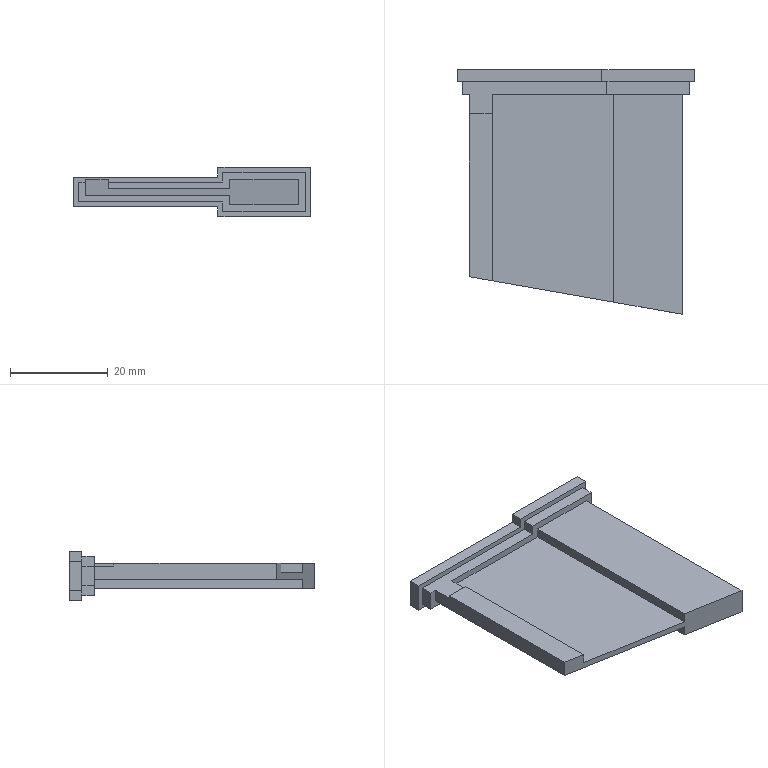Part | SolidWorks | features ICE 4, Extrusion 1 | 1 solid | 31 faces | box 48.36 x 50 x 10.06 mm | volume 6665 mm3 | plane 31
STEP:
#1=CARTESIAN_POINT('',(-43.58,41.,-0.61));
#2=VERTEX_POINT('',#1);
#3=CARTESIAN_POINT('',(-43.58,41.,0.));
#4=VERTEX_POINT('',#3);
#5=CARTESIAN_POINT('',(-43.58,41.,-0.61));
#6=DIRECTION('',(0.,0.,1.));
#7=VECTOR('',#6,1000.);
#8=LINE('',#5,#7);
#9=EDGE_CURVE('',#2,#4,#8,.T.);
#10=ORIENTED_EDGE('',*,*,#9,.F.);
#11=CARTESIAN_POINT('',(-43.58,45.,-0.61));
#12=VERTEX_POINT('',#11);
#13=CARTESIAN_POINT('',(-43.58,45.,-0.61));
#14=DIRECTION('',(0.,-1.,0.));
#15=VECTOR('',#14,1000.);
#16=LINE('',#13,#15);
#17=EDGE_CURVE('',#12,#2,#16,.T.);
#18=ORIENTED_EDGE('',*,*,#17,.F.);
#19=CARTESIAN_POINT('',(-43.58,45.,-3.28));
#20=VERTEX_POINT('',#19);
#21=CARTESIAN_POINT('',(-43.58,45.,-3.28));
#22=DIRECTION('',(0.,0.,1.));
#23=VECTOR('',#22,1000.);
#24=LINE('',#21,#23);
#25=EDGE_CURVE('',#20,#12,#24,.T.);
#26=ORIENTED_EDGE('',*,*,#25,.F.);
#27=CARTESIAN_POINT('',(-43.58,7.684,-3.28));
#28=VERTEX_POINT('',#27);
#29=CARTESIAN_POINT('',(-43.58,45.,-3.28));
#30=DIRECTION('',(0.,-1.,0.));
#31=VECTOR('',#30,1000.);
#32=LINE('',#29,#31);
#33=EDGE_CURVE('',#20,#28,#32,.T.);
#34=ORIENTED_EDGE('',*,*,#33,.T.);
#35=CARTESIAN_POINT('',(-43.58,7.684,0.));
#36=VERTEX_POINT('',#35);
#37=CARTESIAN_POINT('',(-43.58,7.684,-5.28));
#38=DIRECTION('',(0.,0.,1.));
#39=VECTOR('',#38,1000.);
#40=LINE('',#37,#39);
#41=EDGE_CURVE('',#28,#36,#40,.T.);
#42=ORIENTED_EDGE('',*,*,#41,.T.);
#43=CARTESIAN_POINT('',(-43.58,45.,0.));
#44=DIRECTION('',(0.,-1.,0.));
#45=VECTOR('',#44,1000.);
#46=LINE('',#43,#45);
#47=EDGE_CURVE('',#4,#36,#46,.T.);
#48=ORIENTED_EDGE('',*,*,#47,.F.);
#49=EDGE_LOOP('',(#10,#18,#26,#34,#42,#48));
#50=FACE_OUTER_BOUND('',#49,.T.);
#51=CARTESIAN_POINT('',(-43.58,45.,-3.28));
#52=DIRECTION('',(1.,0.,0.));
#53=DIRECTION('',(0.,0.,-1.));
#54=AXIS2_PLACEMENT_3D('',#51,#52,#53);
#55=PLANE('',#54);
#56=ADVANCED_FACE('',(#50),#55,.F.);
#57=CARTESIAN_POINT('',(-38.89,41.,0.));
#58=VERTEX_POINT('',#57);
#59=CARTESIAN_POINT('',(-38.89,6.857,0.));
#60=VERTEX_POINT('',#59);
#61=CARTESIAN_POINT('',(-38.89,45.,0.));
#62=DIRECTION('',(0.,-1.,0.));
#63=VECTOR('',#62,1000.);
#64=LINE('',#61,#63);
#65=EDGE_CURVE('',#58,#60,#64,.T.);
#66=ORIENTED_EDGE('',*,*,#65,.F.);
#67=CARTESIAN_POINT('',(-33.58,41.,0.));
#68=DIRECTION('',(-1.,0.,0.));
#69=VECTOR('',#68,1000.);
#70=LINE('',#67,#69);
#71=EDGE_CURVE('',#58,#4,#70,.T.);
#72=ORIENTED_EDGE('',*,*,#71,.T.);
#73=ORIENTED_EDGE('',*,*,#47,.T.);
#74=CARTESIAN_POINT('',(-43.58,7.684,0.));
#75=DIRECTION('',(-0.9848,0.1736,0.));
#76=VECTOR('',#75,1000.);
#77=LINE('',#74,#76);
#78=EDGE_CURVE('',#60,#36,#77,.T.);
#79=ORIENTED_EDGE('',*,*,#78,.F.);
#80=EDGE_LOOP('',(#66,#72,#73,#79));
#81=FACE_OUTER_BOUND('',#80,.T.);
#82=CARTESIAN_POINT('',(-43.58,45.,0.));
#83=DIRECTION('',(0.,0.,-1.));
#84=DIRECTION('',(-1.,0.,0.));
#85=AXIS2_PLACEMENT_3D('',#82,#83,#84);
#86=PLANE('',#85);
#87=ADVANCED_FACE('',(#81),#86,.F.);
#88=CARTESIAN_POINT('',(-38.89,45.,-0.61));
#89=VERTEX_POINT('',#88);
#90=CARTESIAN_POINT('',(-38.89,45.,-2.));
#91=VERTEX_POINT('',#90);
#92=CARTESIAN_POINT('',(-38.89,45.,0.));
#93=DIRECTION('',(0.,0.,-1.));
#94=VECTOR('',#93,1000.);
#95=LINE('',#92,#94);
#96=EDGE_CURVE('',#89,#91,#95,.T.);
#97=ORIENTED_EDGE('',*,*,#96,.F.);
#98=CARTESIAN_POINT('',(-38.89,41.,-0.61));
#99=VERTEX_POINT('',#98);
#100=CARTESIAN_POINT('',(-38.89,45.,-0.61));
#101=DIRECTION('',(0.,-1.,0.));
#102=VECTOR('',#101,1000.);
#103=LINE('',#100,#102);
#104=EDGE_CURVE('',#89,#99,#103,.T.);
#105=ORIENTED_EDGE('',*,*,#104,.T.);
#106=CARTESIAN_POINT('',(-38.89,41.,0.));
#107=DIRECTION('',(0.,0.,1.));
#108=VECTOR('',#107,1000.);
#109=LINE('',#106,#108);
#110=EDGE_CURVE('',#99,#58,#109,.T.);
#111=ORIENTED_EDGE('',*,*,#110,.T.);
#112=ORIENTED_EDGE('',*,*,#65,.T.);
#113=CARTESIAN_POINT('',(-38.89,6.857,-2.));
#114=VERTEX_POINT('',#113);
#115=CARTESIAN_POINT('',(-38.89,6.857,0.));
#116=DIRECTION('',(0.,0.,-1.));
#117=VECTOR('',#116,1000.);
#118=LINE('',#115,#117);
#119=EDGE_CURVE('',#60,#114,#118,.T.);
#120=ORIENTED_EDGE('',*,*,#119,.T.);
#121=CARTESIAN_POINT('',(-38.89,45.,-2.));
#122=DIRECTION('',(0.,-1.,0.));
#123=VECTOR('',#122,1000.);
#124=LINE('',#121,#123);
#125=EDGE_CURVE('',#91,#114,#124,.T.);
#126=ORIENTED_EDGE('',*,*,#125,.F.);
#127=EDGE_LOOP('',(#97,#105,#111,#112,#120,#126));
#128=FACE_OUTER_BOUND('',#127,.T.);
#129=CARTESIAN_POINT('',(-38.89,45.,0.));
#130=DIRECTION('',(-1.,0.,0.));
#131=DIRECTION('',(0.,0.,1.));
#132=AXIS2_PLACEMENT_3D('',#129,#130,#131);
#133=PLANE('',#132);
#134=ADVANCED_FACE('',(#128),#133,.F.);
#135=ORIENTED_EDGE('',*,*,#125,.T.);
#136=CARTESIAN_POINT('',(-14.09,2.484,-2.));
#137=VERTEX_POINT('',#136);
#138=CARTESIAN_POINT('',(-45.413,8.007,-2.));
#139=DIRECTION('',(0.9848,-0.1736,0.));
#140=VECTOR('',#139,1000.);
#141=LINE('',#138,#140);
#142=EDGE_CURVE('',#114,#137,#141,.T.);
#143=ORIENTED_EDGE('',*,*,#142,.T.);
#144=CARTESIAN_POINT('',(-14.09,45.,-2.));
#145=VERTEX_POINT('',#144);
#146=CARTESIAN_POINT('',(-14.09,45.,-2.));
#147=DIRECTION('',(0.,-1.,0.));
#148=VECTOR('',#147,1000.);
#149=LINE('',#146,#148);
#150=EDGE_CURVE('',#145,#137,#149,.T.);
#151=ORIENTED_EDGE('',*,*,#150,.F.);
#152=CARTESIAN_POINT('',(-38.89,45.,-2.));
#153=DIRECTION('',(1.,0.,0.));
#154=VECTOR('',#153,1000.);
#155=LINE('',#152,#154);
#156=EDGE_CURVE('',#91,#145,#155,.T.);
#157=ORIENTED_EDGE('',*,*,#156,.F.);
#158=EDGE_LOOP('',(#135,#143,#151,#157));
#159=FACE_OUTER_BOUND('',#158,.T.);
#160=CARTESIAN_POINT('',(-38.89,45.,-2.));
#161=DIRECTION('',(0.,0.,-1.));
#162=DIRECTION('',(-1.,0.,0.));
#163=AXIS2_PLACEMENT_3D('',#160,#161,#162);
#164=PLANE('',#163);
#165=ADVANCED_FACE('',(#159),#164,.F.);
#166=ORIENTED_EDGE('',*,*,#150,.T.);
#167=CARTESIAN_POINT('',(-14.09,2.484,0.));
#168=VERTEX_POINT('',#167);
#169=CARTESIAN_POINT('',(-14.09,2.484,-2.));
#170=DIRECTION('',(0.,0.,1.));
#171=VECTOR('',#170,1000.);
#172=LINE('',#169,#171);
#173=EDGE_CURVE('',#137,#168,#172,.T.);
#174=ORIENTED_EDGE('',*,*,#173,.T.);
#175=CARTESIAN_POINT('',(-14.09,45.,0.));
#176=VERTEX_POINT('',#175);
#177=CARTESIAN_POINT('',(-14.09,45.,0.));
#178=DIRECTION('',(0.,-1.,0.));
#179=VECTOR('',#178,1000.);
#180=LINE('',#177,#179);
#181=EDGE_CURVE('',#176,#168,#180,.T.);
#182=ORIENTED_EDGE('',*,*,#181,.F.);
#183=CARTESIAN_POINT('',(-14.09,45.,-2.));
#184=DIRECTION('',(0.,0.,1.));
#185=VECTOR('',#184,1000.);
#186=LINE('',#183,#185);
#187=EDGE_CURVE('',#145,#176,#186,.T.);
#188=ORIENTED_EDGE('',*,*,#187,.F.);
#189=EDGE_LOOP('',(#166,#174,#182,#188));
#190=FACE_OUTER_BOUND('',#189,.T.);
#191=CARTESIAN_POINT('',(-14.09,45.,-2.));
#192=DIRECTION('',(1.,0.,0.));
#193=DIRECTION('',(0.,0.,-1.));
#194=AXIS2_PLACEMENT_3D('',#191,#192,#193);
#195=PLANE('',#194);
#196=ADVANCED_FACE('',(#190),#195,.F.);
#197=ORIENTED_EDGE('',*,*,#181,.T.);
#198=CARTESIAN_POINT('',(0.,0.,0.));
#199=VERTEX_POINT('',#198);
#200=CARTESIAN_POINT('',(-43.58,7.684,0.));
#201=DIRECTION('',(-0.9848,0.1736,0.));
#202=VECTOR('',#201,1000.);
#203=LINE('',#200,#202);
#204=EDGE_CURVE('',#199,#168,#203,.T.);
#205=ORIENTED_EDGE('',*,*,#204,.F.);
#206=CARTESIAN_POINT('',(0.,45.,0.));
#207=VERTEX_POINT('',#206);
#208=CARTESIAN_POINT('',(0.,45.,0.));
#209=DIRECTION('',(0.,-1.,0.));
#210=VECTOR('',#209,1000.);
#211=LINE('',#208,#210);
#212=EDGE_CURVE('',#207,#199,#211,.T.);
#213=ORIENTED_EDGE('',*,*,#212,.F.);
#214=CARTESIAN_POINT('',(-14.09,45.,0.));
#215=DIRECTION('',(1.,0.,0.));
#216=VECTOR('',#215,1000.);
#217=LINE('',#214,#216);
#218=EDGE_CURVE('',#176,#207,#217,.T.);
#219=ORIENTED_EDGE('',*,*,#218,.F.);
#220=EDGE_LOOP('',(#197,#205,#213,#219));
#221=FACE_OUTER_BOUND('',#220,.T.);
#222=CARTESIAN_POINT('',(-14.09,45.,0.));
#223=DIRECTION('',(0.,0.,-1.));
#224=DIRECTION('',(-1.,0.,0.));
#225=AXIS2_PLACEMENT_3D('',#222,#223,#224);
#226=PLANE('',#225);
#227=ADVANCED_FACE('',(#221),#226,.F.);
#228=CARTESIAN_POINT('',(0.,0.,-5.28));
#229=VERTEX_POINT('',#228);
#230=CARTESIAN_POINT('',(0.,0.,0.));
#231=DIRECTION('',(0.,0.,-1.));
#232=VECTOR('',#231,1000.);
#233=LINE('',#230,#232);
#234=EDGE_CURVE('',#199,#229,#233,.T.);
#235=ORIENTED_EDGE('',*,*,#234,.T.);
#236=CARTESIAN_POINT('',(0.,45.,-5.28));
#237=VERTEX_POINT('',#236);
#238=CARTESIAN_POINT('',(0.,45.,-5.28));
#239=DIRECTION('',(0.,-1.,0.));
#240=VECTOR('',#239,1000.);
#241=LINE('',#238,#240);
#242=EDGE_CURVE('',#237,#229,#241,.T.);
#243=ORIENTED_EDGE('',*,*,#242,.F.);
#244=CARTESIAN_POINT('',(0.,45.,0.));
#245=DIRECTION('',(0.,0.,-1.));
#246=VECTOR('',#245,1000.);
#247=LINE('',#244,#246);
#248=EDGE_CURVE('',#207,#237,#247,.T.);
#249=ORIENTED_EDGE('',*,*,#248,.F.);
#250=ORIENTED_EDGE('',*,*,#212,.T.);
#251=EDGE_LOOP('',(#235,#243,#249,#250));
#252=FACE_OUTER_BOUND('',#251,.T.);
#253=CARTESIAN_POINT('',(0.,45.,0.));
#254=DIRECTION('',(-1.,0.,0.));
#255=DIRECTION('',(0.,0.,1.));
#256=AXIS2_PLACEMENT_3D('',#253,#254,#255);
#257=PLANE('',#256);
#258=ADVANCED_FACE('',(#252),#257,.F.);
#259=ORIENTED_EDGE('',*,*,#242,.T.);
#260=CARTESIAN_POINT('',(-14.09,2.484,-5.28));
#261=VERTEX_POINT('',#260);
#262=CARTESIAN_POINT('',(-43.58,7.684,-5.28));
#263=DIRECTION('',(-0.9848,0.1736,0.));
#264=VECTOR('',#263,1000.);
#265=LINE('',#262,#264);
#266=EDGE_CURVE('',#229,#261,#265,.T.);
#267=ORIENTED_EDGE('',*,*,#266,.T.);
#268=CARTESIAN_POINT('',(-14.09,45.,-5.28));
#269=VERTEX_POINT('',#268);
#270=CARTESIAN_POINT('',(-14.09,45.,-5.28));
#271=DIRECTION('',(0.,-1.,0.));
#272=VECTOR('',#271,1000.);
#273=LINE('',#270,#272);
#274=EDGE_CURVE('',#269,#261,#273,.T.);
#275=ORIENTED_EDGE('',*,*,#274,.F.);
#276=CARTESIAN_POINT('',(0.,45.,-5.28));
#277=DIRECTION('',(-1.,0.,0.));
#278=VECTOR('',#277,1000.);
#279=LINE('',#276,#278);
#280=EDGE_CURVE('',#237,#269,#279,.T.);
#281=ORIENTED_EDGE('',*,*,#280,.F.);
#282=EDGE_LOOP('',(#259,#267,#275,#281));
#283=FACE_OUTER_BOUND('',#282,.T.);
#284=CARTESIAN_POINT('',(0.,45.,-5.28));
#285=DIRECTION('',(0.,0.,1.));
#286=DIRECTION('',(1.,0.,0.));
#287=AXIS2_PLACEMENT_3D('',#284,#285,#286);
#288=PLANE('',#287);
#289=ADVANCED_FACE('',(#283),#288,.F.);
#290=ORIENTED_EDGE('',*,*,#274,.T.);
#291=CARTESIAN_POINT('',(-14.09,2.484,-3.28));
#292=VERTEX_POINT('',#291);
#293=CARTESIAN_POINT('',(-14.09,2.484,-5.28));
#294=DIRECTION('',(0.,0.,1.));
#295=VECTOR('',#294,1000.);
#296=LINE('',#293,#295);
#297=EDGE_CURVE('',#261,#292,#296,.T.);
#298=ORIENTED_EDGE('',*,*,#297,.T.);
#299=CARTESIAN_POINT('',(-14.09,45.,-3.28));
#300=VERTEX_POINT('',#299);
#301=CARTESIAN_POINT('',(-14.09,45.,-3.28));
#302=DIRECTION('',(0.,-1.,0.));
#303=VECTOR('',#302,1000.);
#304=LINE('',#301,#303);
#305=EDGE_CURVE('',#300,#292,#304,.T.);
#306=ORIENTED_EDGE('',*,*,#305,.F.);
#307=CARTESIAN_POINT('',(-14.09,45.,-5.28));
#308=DIRECTION('',(0.,0.,1.));
#309=VECTOR('',#308,1000.);
#310=LINE('',#307,#309);
#311=EDGE_CURVE('',#269,#300,#310,.T.);
#312=ORIENTED_EDGE('',*,*,#311,.F.);
#313=EDGE_LOOP('',(#290,#298,#306,#312));
#314=FACE_OUTER_BOUND('',#313,.T.);
#315=CARTESIAN_POINT('',(-14.09,45.,-5.28));
#316=DIRECTION('',(1.,0.,0.));
#317=DIRECTION('',(0.,0.,-1.));
#318=AXIS2_PLACEMENT_3D('',#315,#316,#317);
#319=PLANE('',#318);
#320=ADVANCED_FACE('',(#314),#319,.F.);
#321=ORIENTED_EDGE('',*,*,#305,.T.);
#322=CARTESIAN_POINT('',(-21.361,3.766,-3.28));
#323=DIRECTION('',(-0.9848,0.1736,0.));
#324=VECTOR('',#323,1000.);
#325=LINE('',#322,#324);
#326=EDGE_CURVE('',#292,#28,#325,.T.);
#327=ORIENTED_EDGE('',*,*,#326,.T.);
#328=ORIENTED_EDGE('',*,*,#33,.F.);
#329=CARTESIAN_POINT('',(-14.09,45.,-3.28));
#330=DIRECTION('',(-1.,0.,0.));
#331=VECTOR('',#330,1000.);
#332=LINE('',#329,#331);
#333=EDGE_CURVE('',#300,#20,#332,.T.);
#334=ORIENTED_EDGE('',*,*,#333,.F.);
#335=EDGE_LOOP('',(#321,#327,#328,#334));
#336=FACE_OUTER_BOUND('',#335,.T.);
#337=CARTESIAN_POINT('',(-14.09,45.,-3.28));
#338=DIRECTION('',(0.,0.,1.));
#339=DIRECTION('',(1.,0.,0.));
#340=AXIS2_PLACEMENT_3D('',#337,#338,#339);
#341=PLANE('',#340);
#342=ADVANCED_FACE('',(#336),#341,.F.);
#343=ORIENTED_EDGE('',*,*,#78,.T.);
#344=ORIENTED_EDGE('',*,*,#41,.F.);
#345=ORIENTED_EDGE('',*,*,#326,.F.);
#346=ORIENTED_EDGE('',*,*,#297,.F.);
#347=ORIENTED_EDGE('',*,*,#266,.F.);
#348=ORIENTED_EDGE('',*,*,#234,.F.);
#349=ORIENTED_EDGE('',*,*,#204,.T.);
#350=ORIENTED_EDGE('',*,*,#173,.F.);
#351=ORIENTED_EDGE('',*,*,#142,.F.);
#352=ORIENTED_EDGE('',*,*,#119,.F.);
#353=EDGE_LOOP('',(#343,#344,#345,#346,#347,#348,#349,#350,#351,#352));
#354=FACE_OUTER_BOUND('',#353,.T.);
#355=CARTESIAN_POINT('',(-43.58,7.684,-5.28));
#356=DIRECTION('',(0.1736,0.9848,0.));
#357=DIRECTION('',(-0.9848,0.1736,0.));
#358=AXIS2_PLACEMENT_3D('',#355,#356,#357);
#359=PLANE('',#358);
#360=ADVANCED_FACE('',(#354),#359,.F.);
#361=CARTESIAN_POINT('',(-44.97,45.,-0.61));
#362=VERTEX_POINT('',#361);
#363=CARTESIAN_POINT('',(-44.97,45.,-0.61));
#364=DIRECTION('',(1.,0.,0.));
#365=VECTOR('',#364,1000.);
#366=LINE('',#363,#365);
#367=EDGE_CURVE('',#362,#12,#366,.T.);
#368=ORIENTED_EDGE('',*,*,#367,.T.);
#369=ORIENTED_EDGE('',*,*,#17,.T.);
#370=CARTESIAN_POINT('',(-33.58,41.,-0.61));
#371=DIRECTION('',(-1.,0.,0.));
#372=VECTOR('',#371,1000.);
#373=LINE('',#370,#372);
#374=EDGE_CURVE('',#99,#2,#373,.T.);
#375=ORIENTED_EDGE('',*,*,#374,.F.);
#376=ORIENTED_EDGE('',*,*,#104,.F.);
#377=CARTESIAN_POINT('',(-15.48,45.,-0.61));
#378=VERTEX_POINT('',#377);
#379=CARTESIAN_POINT('',(-44.97,45.,-0.61));
#380=DIRECTION('',(1.,0.,0.));
#381=VECTOR('',#380,1000.);
#382=LINE('',#379,#381);
#383=EDGE_CURVE('',#89,#378,#382,.T.);
#384=ORIENTED_EDGE('',*,*,#383,.T.);
#385=CARTESIAN_POINT('',(-15.48,47.5,-0.61));
#386=VERTEX_POINT('',#385);
#387=CARTESIAN_POINT('',(-15.48,47.5,-0.61));
#388=DIRECTION('',(0.,-1.,0.));
#389=VECTOR('',#388,1000.);
#390=LINE('',#387,#389);
#391=EDGE_CURVE('',#386,#378,#390,.T.);
#392=ORIENTED_EDGE('',*,*,#391,.F.);
#393=CARTESIAN_POINT('',(-44.97,47.5,-0.61));
#394=VERTEX_POINT('',#393);
#395=CARTESIAN_POINT('',(-44.97,47.5,-0.61));
#396=DIRECTION('',(1.,0.,0.));
#397=VECTOR('',#396,1000.);
#398=LINE('',#395,#397);
#399=EDGE_CURVE('',#394,#386,#398,.T.);
#400=ORIENTED_EDGE('',*,*,#399,.F.);
#401=CARTESIAN_POINT('',(-44.97,47.5,-0.61));
#402=DIRECTION('',(0.,-1.,0.));
#403=VECTOR('',#402,1000.);
#404=LINE('',#401,#403);
#405=EDGE_CURVE('',#394,#362,#404,.T.);
#406=ORIENTED_EDGE('',*,*,#405,.T.);
#407=EDGE_LOOP('',(#368,#369,#375,#376,#384,#392,#400,#406));
#408=FACE_OUTER_BOUND('',#407,.T.);
#409=CARTESIAN_POINT('',(-44.97,47.5,-0.61));
#410=DIRECTION('',(0.,0.,-1.));
#411=DIRECTION('',(-1.,0.,0.));
#412=AXIS2_PLACEMENT_3D('',#409,#410,#411);
#413=PLANE('',#412);
#414=ADVANCED_FACE('',(#408),#413,.F.);
#415=CARTESIAN_POINT('',(-15.48,45.,1.39));
#416=VERTEX_POINT('',#415);
#417=CARTESIAN_POINT('',(-15.48,45.,-0.61));
#418=DIRECTION('',(0.,0.,1.));
#419=VECTOR('',#418,1000.);
#420=LINE('',#417,#419);
#421=EDGE_CURVE('',#378,#416,#420,.T.);
#422=ORIENTED_EDGE('',*,*,#421,.T.);
#423=CARTESIAN_POINT('',(-15.48,47.5,1.39));
#424=VERTEX_POINT('',#423);
#425=CARTESIAN_POINT('',(-15.48,47.5,1.39));
#426=DIRECTION('',(0.,-1.,0.));
#427=VECTOR('',#426,1000.);
#428=LINE('',#425,#427);
#429=EDGE_CURVE('',#424,#416,#428,.T.);
#430=ORIENTED_EDGE('',*,*,#429,.F.);
#431=CARTESIAN_POINT('',(-15.48,47.5,-0.61));
#432=DIRECTION('',(0.,0.,1.));
#433=VECTOR('',#432,1000.);
#434=LINE('',#431,#433);
#435=EDGE_CURVE('',#386,#424,#434,.T.);
#436=ORIENTED_EDGE('',*,*,#435,.F.);
#437=ORIENTED_EDGE('',*,*,#391,.T.);
#438=EDGE_LOOP('',(#422,#430,#436,#437));
#439=FACE_OUTER_BOUND('',#438,.T.);
#440=CARTESIAN_POINT('',(-15.48,47.5,-0.61));
#441=DIRECTION('',(1.,0.,0.));
#442=DIRECTION('',(0.,0.,-1.));
#443=AXIS2_PLACEMENT_3D('',#440,#441,#442);
#444=PLANE('',#443);
#445=ADVANCED_FACE('',(#439),#444,.F.);
#446=CARTESIAN_POINT('',(1.39,45.,1.39));
#447=VERTEX_POINT('',#446);
#448=CARTESIAN_POINT('',(-15.48,45.,1.39));
#449=DIRECTION('',(1.,0.,0.));
#450=VECTOR('',#449,1000.);
#451=LINE('',#448,#450);
#452=EDGE_CURVE('',#416,#447,#451,.T.);
#453=ORIENTED_EDGE('',*,*,#452,.T.);
#454=CARTESIAN_POINT('',(1.39,47.5,1.39));
#455=VERTEX_POINT('',#454);
#456=CARTESIAN_POINT('',(1.39,47.5,1.39));
#457=DIRECTION('',(0.,-1.,0.));
#458=VECTOR('',#457,1000.);
#459=LINE('',#456,#458);
#460=EDGE_CURVE('',#455,#447,#459,.T.);
#461=ORIENTED_EDGE('',*,*,#460,.F.);
#462=CARTESIAN_POINT('',(-15.48,47.5,1.39));
#463=DIRECTION('',(1.,0.,0.));
#464=VECTOR('',#463,1000.);
#465=LINE('',#462,#464);
#466=EDGE_CURVE('',#424,#455,#465,.T.);
#467=ORIENTED_EDGE('',*,*,#466,.F.);
#468=ORIENTED_EDGE('',*,*,#429,.T.);
#469=EDGE_LOOP('',(#453,#461,#467,#468));
#470=FACE_OUTER_BOUND('',#469,.T.);
#471=CARTESIAN_POINT('',(-15.48,47.5,1.39));
#472=DIRECTION('',(0.,0.,-1.));
#473=DIRECTION('',(-1.,0.,0.));
#474=AXIS2_PLACEMENT_3D('',#471,#472,#473);
#475=PLANE('',#474);
#476=ADVANCED_FACE('',(#470),#475,.F.);
#477=CARTESIAN_POINT('',(1.39,45.,-6.67));
#478=VERTEX_POINT('',#477);
#479=CARTESIAN_POINT('',(1.39,45.,1.39));
#480=DIRECTION('',(0.,0.,-1.));
#481=VECTOR('',#480,1000.);
#482=LINE('',#479,#481);
#483=EDGE_CURVE('',#447,#478,#482,.T.);
#484=ORIENTED_EDGE('',*,*,#483,.T.);
#485=CARTESIAN_POINT('',(1.39,47.5,-6.67));
#486=VERTEX_POINT('',#485);
#487=CARTESIAN_POINT('',(1.39,47.5,-6.67));
#488=DIRECTION('',(0.,-1.,0.));
#489=VECTOR('',#488,1000.);
#490=LINE('',#487,#489);
#491=EDGE_CURVE('',#486,#478,#490,.T.);
#492=ORIENTED_EDGE('',*,*,#491,.F.);
#493=CARTESIAN_POINT('',(1.39,47.5,1.39));
#494=DIRECTION('',(0.,0.,-1.));
#495=VECTOR('',#494,1000.);
#496=LINE('',#493,#495);
#497=EDGE_CURVE('',#455,#486,#496,.T.);
#498=ORIENTED_EDGE('',*,*,#497,.F.);
#499=ORIENTED_EDGE('',*,*,#460,.T.);
#500=EDGE_LOOP('',(#484,#492,#498,#499));
#501=FACE_OUTER_BOUND('',#500,.T.);
#502=CARTESIAN_POINT('',(1.39,47.5,1.39));
#503=DIRECTION('',(-1.,0.,0.));
#504=DIRECTION('',(0.,0.,1.));
#505=AXIS2_PLACEMENT_3D('',#502,#503,#504);
#506=PLANE('',#505);
#507=ADVANCED_FACE('',(#501),#506,.F.);
#508=CARTESIAN_POINT('',(-15.48,45.,-6.67));
#509=VERTEX_POINT('',#508);
#510=CARTESIAN_POINT('',(1.39,45.,-6.67));
#511=DIRECTION('',(-1.,0.,0.));
#512=VECTOR('',#511,1000.);
#513=LINE('',#510,#512);
#514=EDGE_CURVE('',#478,#509,#513,.T.);
#515=ORIENTED_EDGE('',*,*,#514,.T.);
#516=CARTESIAN_POINT('',(-15.48,47.5,-6.67));
#517=VERTEX_POINT('',#516);
#518=CARTESIAN_POINT('',(-15.48,47.5,-6.67));
#519=DIRECTION('',(0.,-1.,0.));
#520=VECTOR('',#519,1000.);
#521=LINE('',#518,#520);
#522=EDGE_CURVE('',#517,#509,#521,.T.);
#523=ORIENTED_EDGE('',*,*,#522,.F.);
#524=CARTESIAN_POINT('',(1.39,47.5,-6.67));
#525=DIRECTION('',(-1.,0.,0.));
#526=VECTOR('',#525,1000.);
#527=LINE('',#524,#526);
#528=EDGE_CURVE('',#486,#517,#527,.T.);
#529=ORIENTED_EDGE('',*,*,#528,.F.);
#530=ORIENTED_EDGE('',*,*,#491,.T.);
#531=EDGE_LOOP('',(#515,#523,#529,#530));
#532=FACE_OUTER_BOUND('',#531,.T.);
#533=CARTESIAN_POINT('',(1.39,47.5,-6.67));
#534=DIRECTION('',(0.,0.,1.));
#535=DIRECTION('',(1.,0.,0.));
#536=AXIS2_PLACEMENT_3D('',#533,#534,#535);
#537=PLANE('',#536);
#538=ADVANCED_FACE('',(#532),#537,.F.);
#539=CARTESIAN_POINT('',(-15.48,45.,-4.67));
#540=VERTEX_POINT('',#539);
#541=CARTESIAN_POINT('',(-15.48,45.,-6.67));
#542=DIRECTION('',(0.,0.,1.));
#543=VECTOR('',#542,1000.);
#544=LINE('',#541,#543);
#545=EDGE_CURVE('',#509,#540,#544,.T.);
#546=ORIENTED_EDGE('',*,*,#545,.T.);
#547=CARTESIAN_POINT('',(-15.48,47.5,-4.67));
#548=VERTEX_POINT('',#547);
#549=CARTESIAN_POINT('',(-15.48,47.5,-4.67));
#550=DIRECTION('',(0.,-1.,0.));
#551=VECTOR('',#550,1000.);
#552=LINE('',#549,#551);
#553=EDGE_CURVE('',#548,#540,#552,.T.);
#554=ORIENTED_EDGE('',*,*,#553,.F.);
#555=CARTESIAN_POINT('',(-15.48,47.5,-6.67));
#556=DIRECTION('',(0.,0.,1.));
#557=VECTOR('',#556,1000.);
#558=LINE('',#555,#557);
#559=EDGE_CURVE('',#517,#548,#558,.T.);
#560=ORIENTED_EDGE('',*,*,#559,.F.);
#561=ORIENTED_EDGE('',*,*,#522,.T.);
#562=EDGE_LOOP('',(#546,#554,#560,#561));
#563=FACE_OUTER_BOUND('',#562,.T.);
#564=CARTESIAN_POINT('',(-15.48,47.5,-6.67));
#565=DIRECTION('',(1.,0.,0.));
#566=DIRECTION('',(0.,0.,-1.));
#567=AXIS2_PLACEMENT_3D('',#564,#565,#566);
#568=PLANE('',#567);
#569=ADVANCED_FACE('',(#563),#568,.F.);
#570=CARTESIAN_POINT('',(-44.97,45.,-4.67));
#571=VERTEX_POINT('',#570);
#572=CARTESIAN_POINT('',(-15.48,45.,-4.67));
#573=DIRECTION('',(-1.,0.,0.));
#574=VECTOR('',#573,1000.);
#575=LINE('',#572,#574);
#576=EDGE_CURVE('',#540,#571,#575,.T.);
#577=ORIENTED_EDGE('',*,*,#576,.T.);
#578=CARTESIAN_POINT('',(-44.97,47.5,-4.67));
#579=VERTEX_POINT('',#578);
#580=CARTESIAN_POINT('',(-44.97,47.5,-4.67));
#581=DIRECTION('',(0.,-1.,0.));
#582=VECTOR('',#581,1000.);
#583=LINE('',#580,#582);
#584=EDGE_CURVE('',#579,#571,#583,.T.);
#585=ORIENTED_EDGE('',*,*,#584,.F.);
#586=CARTESIAN_POINT('',(-15.48,47.5,-4.67));
#587=DIRECTION('',(-1.,0.,0.));
#588=VECTOR('',#587,1000.);
#589=LINE('',#586,#588);
#590=EDGE_CURVE('',#548,#579,#589,.T.);
#591=ORIENTED_EDGE('',*,*,#590,.F.);
#592=ORIENTED_EDGE('',*,*,#553,.T.);
#593=EDGE_LOOP('',(#577,#585,#591,#592));
#594=FACE_OUTER_BOUND('',#593,.T.);
#595=CARTESIAN_POINT('',(-15.48,47.5,-4.67));
#596=DIRECTION('',(0.,0.,1.));
#597=DIRECTION('',(1.,0.,0.));
#598=AXIS2_PLACEMENT_3D('',#595,#596,#597);
#599=PLANE('',#598);
#600=ADVANCED_FACE('',(#594),#599,.F.);
#601=CARTESIAN_POINT('',(-44.97,45.,-4.67));
#602=DIRECTION('',(0.,0.,1.));
#603=VECTOR('',#602,1000.);
#604=LINE('',#601,#603);
#605=EDGE_CURVE('',#571,#362,#604,.T.);
#606=ORIENTED_EDGE('',*,*,#605,.T.);
#607=ORIENTED_EDGE('',*,*,#405,.F.);
#608=CARTESIAN_POINT('',(-44.97,47.5,-4.67));
#609=DIRECTION('',(0.,0.,1.));
#610=VECTOR('',#609,1000.);
#611=LINE('',#608,#610);
#612=EDGE_CURVE('',#579,#394,#611,.T.);
#613=ORIENTED_EDGE('',*,*,#612,.F.);
#614=ORIENTED_EDGE('',*,*,#584,.T.);
#615=EDGE_LOOP('',(#606,#607,#613,#614));
#616=FACE_OUTER_BOUND('',#615,.T.);
#617=CARTESIAN_POINT('',(-44.97,47.5,-4.67));
#618=DIRECTION('',(1.,0.,0.));
#619=DIRECTION('',(0.,0.,-1.));
#620=AXIS2_PLACEMENT_3D('',#617,#618,#619);
#621=PLANE('',#620);
#622=ADVANCED_FACE('',(#616),#621,.F.);
#623=ORIENTED_EDGE('',*,*,#333,.T.);
#624=ORIENTED_EDGE('',*,*,#25,.T.);
#625=ORIENTED_EDGE('',*,*,#367,.F.);
#626=ORIENTED_EDGE('',*,*,#605,.F.);
#627=ORIENTED_EDGE('',*,*,#576,.F.);
#628=ORIENTED_EDGE('',*,*,#545,.F.);
#629=ORIENTED_EDGE('',*,*,#514,.F.);
#630=ORIENTED_EDGE('',*,*,#483,.F.);
#631=ORIENTED_EDGE('',*,*,#452,.F.);
#632=ORIENTED_EDGE('',*,*,#421,.F.);
#633=ORIENTED_EDGE('',*,*,#383,.F.);
#634=ORIENTED_EDGE('',*,*,#96,.T.);
#635=ORIENTED_EDGE('',*,*,#156,.T.);
#636=ORIENTED_EDGE('',*,*,#187,.T.);
#637=ORIENTED_EDGE('',*,*,#218,.T.);
#638=ORIENTED_EDGE('',*,*,#248,.T.);
#639=ORIENTED_EDGE('',*,*,#280,.T.);
#640=ORIENTED_EDGE('',*,*,#311,.T.);
#641=EDGE_LOOP('',(#623,#624,#625,#626,#627,#628,#629,#630,#631,#632,#633,#634,#635,#636,#637,#638,#639,#640));
#642=FACE_OUTER_BOUND('',#641,.T.);
#643=CARTESIAN_POINT('',(0.,45.,0.));
#644=DIRECTION('',(0.,-1.,0.));
#645=DIRECTION('',(0.,0.,-1.));
#646=AXIS2_PLACEMENT_3D('',#643,#644,#645);
#647=PLANE('',#646);
#648=ADVANCED_FACE('',(#642),#647,.T.);
#649=CARTESIAN_POINT('',(-45.97,47.5,0.39));
#650=VERTEX_POINT('',#649);
#651=CARTESIAN_POINT('',(-16.48,47.5,0.39));
#652=VERTEX_POINT('',#651);
#653=CARTESIAN_POINT('',(-45.97,47.5,0.39));
#654=DIRECTION('',(1.,0.,0.));
#655=VECTOR('',#654,1000.);
#656=LINE('',#653,#655);
#657=EDGE_CURVE('',#650,#652,#656,.T.);
#658=ORIENTED_EDGE('',*,*,#657,.F.);
#659=CARTESIAN_POINT('',(-45.97,47.5,-5.67));
#660=VERTEX_POINT('',#659);
#661=CARTESIAN_POINT('',(-45.97,47.5,-5.67));
#662=DIRECTION('',(0.,0.,1.));
#663=VECTOR('',#662,1000.);
#664=LINE('',#661,#663);
#665=EDGE_CURVE('',#660,#650,#664,.T.);
#666=ORIENTED_EDGE('',*,*,#665,.F.);
#667=CARTESIAN_POINT('',(-16.48,47.5,-5.67));
#668=VERTEX_POINT('',#667);
#669=CARTESIAN_POINT('',(-16.48,47.5,-5.67));
#670=DIRECTION('',(-1.,0.,0.));
#671=VECTOR('',#670,1000.);
#672=LINE('',#669,#671);
#673=EDGE_CURVE('',#668,#660,#672,.T.);
#674=ORIENTED_EDGE('',*,*,#673,.F.);
#675=CARTESIAN_POINT('',(-16.48,47.5,-7.67));
#676=VERTEX_POINT('',#675);
#677=CARTESIAN_POINT('',(-16.48,47.5,-7.67));
#678=DIRECTION('',(0.,0.,1.));
#679=VECTOR('',#678,1000.);
#680=LINE('',#677,#679);
#681=EDGE_CURVE('',#676,#668,#680,.T.);
#682=ORIENTED_EDGE('',*,*,#681,.F.);
#683=CARTESIAN_POINT('',(2.39,47.5,-7.67));
#684=VERTEX_POINT('',#683);
#685=CARTESIAN_POINT('',(2.39,47.5,-7.67));
#686=DIRECTION('',(-1.,0.,0.));
#687=VECTOR('',#686,1000.);
#688=LINE('',#685,#687);
#689=EDGE_CURVE('',#684,#676,#688,.T.);
#690=ORIENTED_EDGE('',*,*,#689,.F.);
#691=CARTESIAN_POINT('',(2.39,47.5,2.39));
#692=VERTEX_POINT('',#691);
#693=CARTESIAN_POINT('',(2.39,47.5,2.39));
#694=DIRECTION('',(0.,0.,-1.));
#695=VECTOR('',#694,1000.);
#696=LINE('',#693,#695);
#697=EDGE_CURVE('',#692,#684,#696,.T.);
#698=ORIENTED_EDGE('',*,*,#697,.F.);
#699=CARTESIAN_POINT('',(-16.48,47.5,2.39));
#700=VERTEX_POINT('',#699);
#701=CARTESIAN_POINT('',(-16.48,47.5,2.39));
#702=DIRECTION('',(1.,0.,0.));
#703=VECTOR('',#702,1000.);
#704=LINE('',#701,#703);
#705=EDGE_CURVE('',#700,#692,#704,.T.);
#706=ORIENTED_EDGE('',*,*,#705,.F.);
#707=CARTESIAN_POINT('',(-16.48,47.5,0.39));
#708=DIRECTION('',(0.,0.,1.));
#709=VECTOR('',#708,1000.);
#710=LINE('',#707,#709);
#711=EDGE_CURVE('',#652,#700,#710,.T.);
#712=ORIENTED_EDGE('',*,*,#711,.F.);
#713=EDGE_LOOP('',(#658,#666,#674,#682,#690,#698,#706,#712));
#714=FACE_OUTER_BOUND('',#713,.T.);
#715=ORIENTED_EDGE('',*,*,#399,.T.);
#716=ORIENTED_EDGE('',*,*,#435,.T.);
#717=ORIENTED_EDGE('',*,*,#466,.T.);
#718=ORIENTED_EDGE('',*,*,#497,.T.);
#719=ORIENTED_EDGE('',*,*,#528,.T.);
#720=ORIENTED_EDGE('',*,*,#559,.T.);
#721=ORIENTED_EDGE('',*,*,#590,.T.);
#722=ORIENTED_EDGE('',*,*,#612,.T.);
#723=EDGE_LOOP('',(#715,#716,#717,#718,#719,#720,#721,#722));
#724=FACE_BOUND('',#723,.T.);
#725=CARTESIAN_POINT('',(0.,47.5,0.));
#726=DIRECTION('',(0.,-1.,0.));
#727=DIRECTION('',(0.,0.,-1.));
#728=AXIS2_PLACEMENT_3D('',#725,#726,#727);
#729=PLANE('',#728);
#730=ADVANCED_FACE('',(#714,#724),#729,.T.);
#731=ORIENTED_EDGE('',*,*,#657,.T.);
#732=CARTESIAN_POINT('',(-16.48,50.,0.39));
#733=VERTEX_POINT('',#732);
#734=CARTESIAN_POINT('',(-16.48,50.,0.39));
#735=DIRECTION('',(0.,-1.,0.));
#736=VECTOR('',#735,1000.);
#737=LINE('',#734,#736);
#738=EDGE_CURVE('',#733,#652,#737,.T.);
#739=ORIENTED_EDGE('',*,*,#738,.F.);
#740=CARTESIAN_POINT('',(-45.97,50.,0.39));
#741=VERTEX_POINT('',#740);
#742=CARTESIAN_POINT('',(-45.97,50.,0.39));
#743=DIRECTION('',(1.,0.,0.));
#744=VECTOR('',#743,1000.);
#745=LINE('',#742,#744);
#746=EDGE_CURVE('',#741,#733,#745,.T.);
#747=ORIENTED_EDGE('',*,*,#746,.F.);
#748=CARTESIAN_POINT('',(-45.97,50.,0.39));
#749=DIRECTION('',(0.,-1.,0.));
#750=VECTOR('',#749,1000.);
#751=LINE('',#748,#750);
#752=EDGE_CURVE('',#741,#650,#751,.T.);
#753=ORIENTED_EDGE('',*,*,#752,.T.);
#754=EDGE_LOOP('',(#731,#739,#747,#753));
#755=FACE_OUTER_BOUND('',#754,.T.);
#756=CARTESIAN_POINT('',(-45.97,50.,0.39));
#757=DIRECTION('',(0.,0.,-1.));
#758=DIRECTION('',(-1.,0.,0.));
#759=AXIS2_PLACEMENT_3D('',#756,#757,#758);
#760=PLANE('',#759);
#761=ADVANCED_FACE('',(#755),#760,.F.);
#762=ORIENTED_EDGE('',*,*,#711,.T.);
#763=CARTESIAN_POINT('',(-16.48,50.,2.39));
#764=VERTEX_POINT('',#763);
#765=CARTESIAN_POINT('',(-16.48,50.,2.39));
#766=DIRECTION('',(0.,-1.,0.));
#767=VECTOR('',#766,1000.);
#768=LINE('',#765,#767);
#769=EDGE_CURVE('',#764,#700,#768,.T.);
#770=ORIENTED_EDGE('',*,*,#769,.F.);
#771=CARTESIAN_POINT('',(-16.48,50.,0.39));
#772=DIRECTION('',(0.,0.,1.));
#773=VECTOR('',#772,1000.);
#774=LINE('',#771,#773);
#775=EDGE_CURVE('',#733,#764,#774,.T.);
#776=ORIENTED_EDGE('',*,*,#775,.F.);
#777=ORIENTED_EDGE('',*,*,#738,.T.);
#778=EDGE_LOOP('',(#762,#770,#776,#777));
#779=FACE_OUTER_BOUND('',#778,.T.);
#780=CARTESIAN_POINT('',(-16.48,50.,0.39));
#781=DIRECTION('',(1.,0.,0.));
#782=DIRECTION('',(0.,0.,-1.));
#783=AXIS2_PLACEMENT_3D('',#780,#781,#782);
#784=PLANE('',#783);
#785=ADVANCED_FACE('',(#779),#784,.F.);
#786=ORIENTED_EDGE('',*,*,#705,.T.);
#787=CARTESIAN_POINT('',(2.39,50.,2.39));
#788=VERTEX_POINT('',#787);
#789=CARTESIAN_POINT('',(2.39,50.,2.39));
#790=DIRECTION('',(0.,-1.,0.));
#791=VECTOR('',#790,1000.);
#792=LINE('',#789,#791);
#793=EDGE_CURVE('',#788,#692,#792,.T.);
#794=ORIENTED_EDGE('',*,*,#793,.F.);
#795=CARTESIAN_POINT('',(-16.48,50.,2.39));
#796=DIRECTION('',(1.,0.,0.));
#797=VECTOR('',#796,1000.);
#798=LINE('',#795,#797);
#799=EDGE_CURVE('',#764,#788,#798,.T.);
#800=ORIENTED_EDGE('',*,*,#799,.F.);
#801=ORIENTED_EDGE('',*,*,#769,.T.);
#802=EDGE_LOOP('',(#786,#794,#800,#801));
#803=FACE_OUTER_BOUND('',#802,.T.);
#804=CARTESIAN_POINT('',(-16.48,50.,2.39));
#805=DIRECTION('',(0.,0.,-1.));
#806=DIRECTION('',(-1.,0.,0.));
#807=AXIS2_PLACEMENT_3D('',#804,#805,#806);
#808=PLANE('',#807);
#809=ADVANCED_FACE('',(#803),#808,.F.);
#810=ORIENTED_EDGE('',*,*,#697,.T.);
#811=CARTESIAN_POINT('',(2.39,50.,-7.67));
#812=VERTEX_POINT('',#811);
#813=CARTESIAN_POINT('',(2.39,50.,-7.67));
#814=DIRECTION('',(0.,-1.,0.));
#815=VECTOR('',#814,1000.);
#816=LINE('',#813,#815);
#817=EDGE_CURVE('',#812,#684,#816,.T.);
#818=ORIENTED_EDGE('',*,*,#817,.F.);
#819=CARTESIAN_POINT('',(2.39,50.,2.39));
#820=DIRECTION('',(0.,0.,-1.));
#821=VECTOR('',#820,1000.);
#822=LINE('',#819,#821);
#823=EDGE_CURVE('',#788,#812,#822,.T.);
#824=ORIENTED_EDGE('',*,*,#823,.F.);
#825=ORIENTED_EDGE('',*,*,#793,.T.);
#826=EDGE_LOOP('',(#810,#818,#824,#825));
#827=FACE_OUTER_BOUND('',#826,.T.);
#828=CARTESIAN_POINT('',(2.39,50.,2.39));
#829=DIRECTION('',(-1.,0.,0.));
#830=DIRECTION('',(0.,0.,1.));
#831=AXIS2_PLACEMENT_3D('',#828,#829,#830);
#832=PLANE('',#831);
#833=ADVANCED_FACE('',(#827),#832,.F.);
#834=ORIENTED_EDGE('',*,*,#689,.T.);
#835=CARTESIAN_POINT('',(-16.48,50.,-7.67));
#836=VERTEX_POINT('',#835);
#837=CARTESIAN_POINT('',(-16.48,50.,-7.67));
#838=DIRECTION('',(0.,-1.,0.));
#839=VECTOR('',#838,1000.);
#840=LINE('',#837,#839);
#841=EDGE_CURVE('',#836,#676,#840,.T.);
#842=ORIENTED_EDGE('',*,*,#841,.F.);
#843=CARTESIAN_POINT('',(2.39,50.,-7.67));
#844=DIRECTION('',(-1.,0.,0.));
#845=VECTOR('',#844,1000.);
#846=LINE('',#843,#845);
#847=EDGE_CURVE('',#812,#836,#846,.T.);
#848=ORIENTED_EDGE('',*,*,#847,.F.);
#849=ORIENTED_EDGE('',*,*,#817,.T.);
#850=EDGE_LOOP('',(#834,#842,#848,#849));
#851=FACE_OUTER_BOUND('',#850,.T.);
#852=CARTESIAN_POINT('',(2.39,50.,-7.67));
#853=DIRECTION('',(0.,0.,1.));
#854=DIRECTION('',(1.,0.,0.));
#855=AXIS2_PLACEMENT_3D('',#852,#853,#854);
#856=PLANE('',#855);
#857=ADVANCED_FACE('',(#851),#856,.F.);
#858=ORIENTED_EDGE('',*,*,#681,.T.);
#859=CARTESIAN_POINT('',(-16.48,50.,-5.67));
#860=VERTEX_POINT('',#859);
#861=CARTESIAN_POINT('',(-16.48,50.,-5.67));
#862=DIRECTION('',(0.,-1.,0.));
#863=VECTOR('',#862,1000.);
#864=LINE('',#861,#863);
#865=EDGE_CURVE('',#860,#668,#864,.T.);
#866=ORIENTED_EDGE('',*,*,#865,.F.);
#867=CARTESIAN_POINT('',(-16.48,50.,-7.67));
#868=DIRECTION('',(0.,0.,1.));
#869=VECTOR('',#868,1000.);
#870=LINE('',#867,#869);
#871=EDGE_CURVE('',#836,#860,#870,.T.);
#872=ORIENTED_EDGE('',*,*,#871,.F.);
#873=ORIENTED_EDGE('',*,*,#841,.T.);
#874=EDGE_LOOP('',(#858,#866,#872,#873));
#875=FACE_OUTER_BOUND('',#874,.T.);
#876=CARTESIAN_POINT('',(-16.48,50.,-7.67));
#877=DIRECTION('',(1.,0.,0.));
#878=DIRECTION('',(0.,0.,-1.));
#879=AXIS2_PLACEMENT_3D('',#876,#877,#878);
#880=PLANE('',#879);
#881=ADVANCED_FACE('',(#875),#880,.F.);
#882=ORIENTED_EDGE('',*,*,#673,.T.);
#883=CARTESIAN_POINT('',(-45.97,50.,-5.67));
#884=VERTEX_POINT('',#883);
#885=CARTESIAN_POINT('',(-45.97,50.,-5.67));
#886=DIRECTION('',(0.,-1.,0.));
#887=VECTOR('',#886,1000.);
#888=LINE('',#885,#887);
#889=EDGE_CURVE('',#884,#660,#888,.T.);
#890=ORIENTED_EDGE('',*,*,#889,.F.);
#891=CARTESIAN_POINT('',(-16.48,50.,-5.67));
#892=DIRECTION('',(-1.,0.,0.));
#893=VECTOR('',#892,1000.);
#894=LINE('',#891,#893);
#895=EDGE_CURVE('',#860,#884,#894,.T.);
#896=ORIENTED_EDGE('',*,*,#895,.F.);
#897=ORIENTED_EDGE('',*,*,#865,.T.);
#898=EDGE_LOOP('',(#882,#890,#896,#897));
#899=FACE_OUTER_BOUND('',#898,.T.);
#900=CARTESIAN_POINT('',(-16.48,50.,-5.67));
#901=DIRECTION('',(0.,0.,1.));
#902=DIRECTION('',(1.,0.,0.));
#903=AXIS2_PLACEMENT_3D('',#900,#901,#902);
#904=PLANE('',#903);
#905=ADVANCED_FACE('',(#899),#904,.F.);
#906=ORIENTED_EDGE('',*,*,#665,.T.);
#907=ORIENTED_EDGE('',*,*,#752,.F.);
#908=CARTESIAN_POINT('',(-45.97,50.,-5.67));
#909=DIRECTION('',(0.,0.,1.));
#910=VECTOR('',#909,1000.);
#911=LINE('',#908,#910);
#912=EDGE_CURVE('',#884,#741,#911,.T.);
#913=ORIENTED_EDGE('',*,*,#912,.F.);
#914=ORIENTED_EDGE('',*,*,#889,.T.);
#915=EDGE_LOOP('',(#906,#907,#913,#914));
#916=FACE_OUTER_BOUND('',#915,.T.);
#917=CARTESIAN_POINT('',(-45.97,50.,-5.67));
#918=DIRECTION('',(1.,0.,0.));
#919=DIRECTION('',(0.,0.,-1.));
#920=AXIS2_PLACEMENT_3D('',#917,#918,#919);
#921=PLANE('',#920);
#922=ADVANCED_FACE('',(#916),#921,.F.);
#923=ORIENTED_EDGE('',*,*,#746,.T.);
#924=ORIENTED_EDGE('',*,*,#775,.T.);
#925=ORIENTED_EDGE('',*,*,#799,.T.);
#926=ORIENTED_EDGE('',*,*,#823,.T.);
#927=ORIENTED_EDGE('',*,*,#847,.T.);
#928=ORIENTED_EDGE('',*,*,#871,.T.);
#929=ORIENTED_EDGE('',*,*,#895,.T.);
#930=ORIENTED_EDGE('',*,*,#912,.T.);
#931=EDGE_LOOP('',(#923,#924,#925,#926,#927,#928,#929,#930));
#932=FACE_OUTER_BOUND('',#931,.T.);
#933=CARTESIAN_POINT('',(0.,50.,0.));
#934=DIRECTION('',(0.,-1.,0.));
#935=DIRECTION('',(0.,0.,-1.));
#936=AXIS2_PLACEMENT_3D('',#933,#934,#935);
#937=PLANE('',#936);
#938=ADVANCED_FACE('',(#932),#937,.F.);
#939=ORIENTED_EDGE('',*,*,#374,.T.);
#940=ORIENTED_EDGE('',*,*,#9,.T.);
#941=ORIENTED_EDGE('',*,*,#71,.F.);
#942=ORIENTED_EDGE('',*,*,#110,.F.);
#943=EDGE_LOOP('',(#939,#940,#941,#942));
#944=FACE_OUTER_BOUND('',#943,.T.);
#945=CARTESIAN_POINT('',(-33.58,41.,-0.61));
#946=DIRECTION('',(0.,-1.,0.));
#947=DIRECTION('',(0.,0.,-1.));
#948=AXIS2_PLACEMENT_3D('',#945,#946,#947);
#949=PLANE('',#948);
#950=ADVANCED_FACE('',(#944),#949,.F.);
#951=CLOSED_SHELL('',(#56,#87,#134,#165,#196,#227,#258,#289,#320,#342,#360,#414,#445,#476,#507,#538,#569,#600,#622,#648,#730,#761,#785,#809,#833,#857,#881,#905,#922,#938,#950));
#952=MANIFOLD_SOLID_BREP('',#951);
#953=CARTESIAN_POINT('',(0.,0.,0.));
#954=DIRECTION('',(0.,0.,1.));
#955=DIRECTION('',(1.,0.,0.));
#956=AXIS2_PLACEMENT_3D('',#953,#954,#955);
#957=(LENGTH_UNIT()NAMED_UNIT(*)SI_UNIT(.MILLI.,.METRE.));
#958=UNCERTAINTY_MEASURE_WITH_UNIT(LENGTH_MEASURE(0.00001),#957,'','');
#959=(NAMED_UNIT(*)PLANE_ANGLE_UNIT()SI_UNIT($,.RADIAN.));
#960=(NAMED_UNIT(*)SI_UNIT($,.STERADIAN.)SOLID_ANGLE_UNIT());
#961=(GEOMETRIC_REPRESENTATION_CONTEXT(3)GLOBAL_UNCERTAINTY_ASSIGNED_CONTEXT((#958))GLOBAL_UNIT_ASSIGNED_CONTEXT((#957,#959,#960))REPRESENTATION_CONTEXT('',''));
#962=ADVANCED_BREP_SHAPE_REPRESENTATION('',(#952,#956),#961);